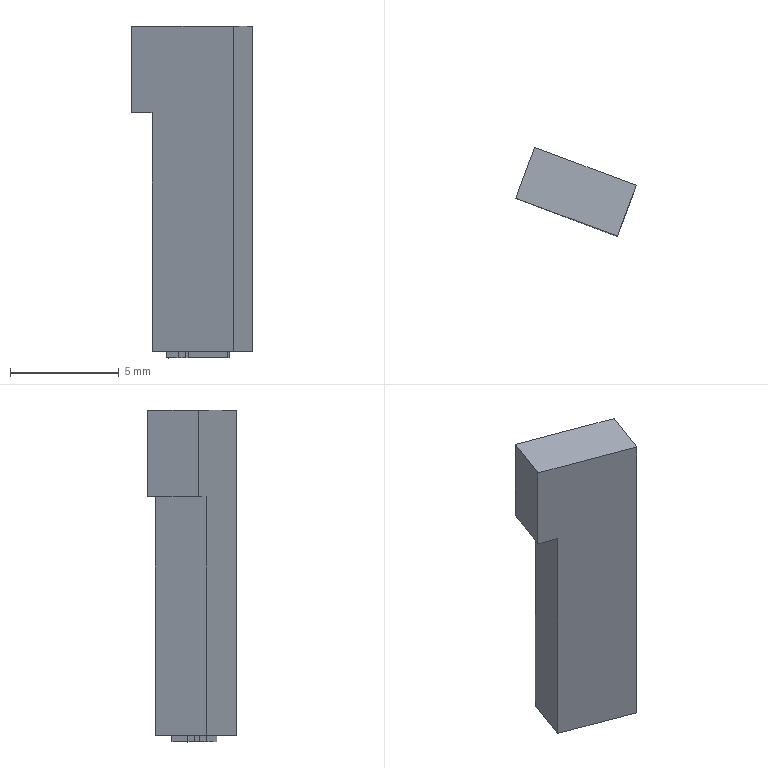Part | NX | features 13 2 | 1 solid | 24 faces | box 5.559 x 4.093 x 15.3 mm | volume 160.547 mm3 | plane 24
STEP:
#1=CARTESIAN_POINT('',(356.25,41.783,0.002111));
#2=VERTEX_POINT('',#1);
#3=CARTESIAN_POINT('',(355.374,39.441,0.002111));
#4=VERTEX_POINT('',#3);
#5=CARTESIAN_POINT('',(359.225,49.741,0.002111));
#6=DIRECTION('',(-0.3502,-0.9367,0.000000001));
#7=VECTOR('',#6,1000.);
#8=LINE('',#5,#7);
#9=EDGE_CURVE('',#2,#4,#8,.T.);
#10=ORIENTED_EDGE('',*,*,#9,.T.);
#11=CARTESIAN_POINT('',(351.627,40.842,0.002031));
#12=VERTEX_POINT('',#11);
#13=CARTESIAN_POINT('',(353.501,40.141,0.002071));
#14=DIRECTION('',(-0.9367,0.3502,-0.00001998));
#15=VECTOR('',#14,1000.);
#16=LINE('',#13,#15);
#17=EDGE_CURVE('',#4,#12,#16,.T.);
#18=ORIENTED_EDGE('',*,*,#17,.T.);
#19=CARTESIAN_POINT('',(352.503,43.183,0.002031));
#20=VERTEX_POINT('',#19);
#21=CARTESIAN_POINT('',(355.478,51.142,0.002031));
#22=DIRECTION('',(0.3502,0.9367,-0.000000001));
#23=VECTOR('',#22,1000.);
#24=LINE('',#21,#23);
#25=EDGE_CURVE('',#12,#20,#24,.T.);
#26=ORIENTED_EDGE('',*,*,#25,.T.);
#27=CARTESIAN_POINT('',(354.376,42.483,0.002071));
#28=DIRECTION('',(0.9367,-0.3502,0.00001998));
#29=VECTOR('',#28,1000.);
#30=LINE('',#27,#29);
#31=EDGE_CURVE('',#20,#2,#30,.T.);
#32=ORIENTED_EDGE('',*,*,#31,.T.);
#33=EDGE_LOOP('',(#10,#18,#26,#32));
#34=FACE_BOUND('',#33,.T.);
#35=CARTESIAN_POINT('',(352.297,41.392,0.00204));
#36=VERTEX_POINT('',#35);
#37=CARTESIAN_POINT('',(352.402,41.672,0.00204));
#38=VERTEX_POINT('',#37);
#39=CARTESIAN_POINT('',(355.885,50.989,0.00204));
#40=DIRECTION('',(0.3502,0.9367,-0.000000001));
#41=VECTOR('',#40,1000.);
#42=LINE('',#39,#41);
#43=EDGE_CURVE('',#36,#38,#42,.T.);
#44=ORIENTED_EDGE('',*,*,#43,.F.);
#45=CARTESIAN_POINT('',(352.97,41.141,0.002054));
#46=VERTEX_POINT('',#45);
#47=CARTESIAN_POINT('',(353.763,40.844,0.002071));
#48=DIRECTION('',(-0.9367,0.3502,-0.00001998));
#49=VECTOR('',#48,1000.);
#50=LINE('',#47,#49);
#51=EDGE_CURVE('',#46,#36,#50,.T.);
#52=ORIENTED_EDGE('',*,*,#51,.F.);
#53=CARTESIAN_POINT('',(352.855,40.833,0.002054));
#54=VERTEX_POINT('',#53);
#55=CARTESIAN_POINT('',(356.558,50.738,0.002054));
#56=DIRECTION('',(0.3502,0.9367,-0.000000001));
#57=VECTOR('',#56,1000.);
#58=LINE('',#55,#57);
#59=EDGE_CURVE('',#54,#46,#58,.T.);
#60=ORIENTED_EDGE('',*,*,#59,.F.);
#61=CARTESIAN_POINT('',(353.171,40.714,0.002061));
#62=VERTEX_POINT('',#61);
#63=CARTESIAN_POINT('',(353.648,40.536,0.002071));
#64=DIRECTION('',(-0.9367,0.3502,-0.00001998));
#65=VECTOR('',#64,1000.);
#66=LINE('',#63,#65);
#67=EDGE_CURVE('',#62,#54,#66,.T.);
#68=ORIENTED_EDGE('',*,*,#67,.F.);
#69=CARTESIAN_POINT('',(353.286,41.022,0.002061));
#70=VERTEX_POINT('',#69);
#71=CARTESIAN_POINT('',(356.874,50.62,0.002061));
#72=DIRECTION('',(-0.3502,-0.9367,0.000000001));
#73=VECTOR('',#72,1000.);
#74=LINE('',#71,#73);
#75=EDGE_CURVE('',#70,#62,#74,.T.);
#76=ORIENTED_EDGE('',*,*,#75,.F.);
#77=CARTESIAN_POINT('',(355.107,40.342,0.0021));
#78=VERTEX_POINT('',#77);
#79=CARTESIAN_POINT('',(353.763,40.844,0.002071));
#80=DIRECTION('',(-0.9367,0.3502,-0.00001998));
#81=VECTOR('',#80,1000.);
#82=LINE('',#79,#81);
#83=EDGE_CURVE('',#78,#70,#82,.T.);
#84=ORIENTED_EDGE('',*,*,#83,.F.);
#85=CARTESIAN_POINT('',(355.192,40.57,0.0021));
#86=VERTEX_POINT('',#85);
#87=CARTESIAN_POINT('',(358.695,49.939,0.0021));
#88=DIRECTION('',(-0.3502,-0.9367,0.000000001));
#89=VECTOR('',#88,1000.);
#90=LINE('',#87,#89);
#91=EDGE_CURVE('',#86,#78,#90,.T.);
#92=ORIENTED_EDGE('',*,*,#91,.F.);
#93=CARTESIAN_POINT('',(353.761,42.291,0.002061));
#94=VERTEX_POINT('',#93);
#95=CARTESIAN_POINT('',(351.223,45.342,0.001992));
#96=DIRECTION('',(0.6395,-0.7688,0.00001735));
#97=VECTOR('',#96,1000.);
#98=LINE('',#95,#97);
#99=EDGE_CURVE('',#94,#86,#98,.T.);
#100=ORIENTED_EDGE('',*,*,#99,.F.);
#101=CARTESIAN_POINT('',(353.444,42.41,0.002054));
#102=VERTEX_POINT('',#101);
#103=CARTESIAN_POINT('',(354.238,42.113,0.002071));
#104=DIRECTION('',(0.9367,-0.3502,0.00001998));
#105=VECTOR('',#104,1000.);
#106=LINE('',#103,#105);
#107=EDGE_CURVE('',#102,#94,#106,.T.);
#108=ORIENTED_EDGE('',*,*,#107,.F.);
#109=CARTESIAN_POINT('',(353.075,41.42,0.002054));
#110=VERTEX_POINT('',#109);
#111=CARTESIAN_POINT('',(356.558,50.738,0.002054));
#112=DIRECTION('',(0.3502,0.9367,-0.000000001));
#113=VECTOR('',#112,1000.);
#114=LINE('',#111,#113);
#115=EDGE_CURVE('',#110,#102,#114,.T.);
#116=ORIENTED_EDGE('',*,*,#115,.F.);
#117=CARTESIAN_POINT('',(353.868,41.124,0.002071));
#118=DIRECTION('',(0.9367,-0.3502,0.00001998));
#119=VECTOR('',#118,1000.);
#120=LINE('',#117,#119);
#121=EDGE_CURVE('',#38,#110,#120,.T.);
#122=ORIENTED_EDGE('',*,*,#121,.F.);
#123=EDGE_LOOP('',(#44,#52,#60,#68,#76,#84,#92,#100,#108,#116,#122));
#124=FACE_BOUND('',#123,.T.);
#125=CARTESIAN_POINT('',(357.352,50.441,0.002071));
#126=DIRECTION('',(-0.00001871,0.000006998,1.));
#127=DIRECTION('',(0.9172,-0.3985,0.00001995));
#128=AXIS2_PLACEMENT_3D('',#125,#126,#127);
#129=PLANE('',#128);
#130=ADVANCED_FACE('',(#34,#124),#129,.F.);
#131=CARTESIAN_POINT('',(351.627,40.842,11.002));
#132=VERTEX_POINT('',#131);
#133=CARTESIAN_POINT('',(352.503,43.184,11.002));
#134=VERTEX_POINT('',#133);
#135=CARTESIAN_POINT('',(352.503,43.184,11.002));
#136=DIRECTION('',(0.3502,0.9367,-0.000000001));
#137=VECTOR('',#136,1000.);
#138=LINE('',#135,#137);
#139=EDGE_CURVE('',#132,#134,#138,.T.);
#140=ORIENTED_EDGE('',*,*,#139,.F.);
#141=CARTESIAN_POINT('',(350.691,41.192,11.002));
#142=VERTEX_POINT('',#141);
#143=CARTESIAN_POINT('',(353.501,40.141,11.002));
#144=DIRECTION('',(-0.9367,0.3502,-0.00001998));
#145=VECTOR('',#144,1000.);
#146=LINE('',#143,#145);
#147=EDGE_CURVE('',#132,#142,#146,.T.);
#148=ORIENTED_EDGE('',*,*,#147,.T.);
#149=CARTESIAN_POINT('',(351.566,43.534,11.002));
#150=VERTEX_POINT('',#149);
#151=CARTESIAN_POINT('',(353.666,49.15,11.002));
#152=DIRECTION('',(-0.3502,-0.9367,0.000000001));
#153=VECTOR('',#152,1000.);
#154=LINE('',#151,#153);
#155=EDGE_CURVE('',#150,#142,#154,.T.);
#156=ORIENTED_EDGE('',*,*,#155,.F.);
#157=CARTESIAN_POINT('',(354.376,42.483,11.002));
#158=DIRECTION('',(-0.9367,0.3502,-0.00001998));
#159=VECTOR('',#158,1000.);
#160=LINE('',#157,#159);
#161=EDGE_CURVE('',#134,#150,#160,.T.);
#162=ORIENTED_EDGE('',*,*,#161,.F.);
#163=EDGE_LOOP('',(#140,#148,#156,#162));
#164=FACE_BOUND('',#163,.T.);
#165=CARTESIAN_POINT('',(356.476,48.1,11.002));
#166=DIRECTION('',(0.00001871,-0.000006998,-1.));
#167=DIRECTION('',(0.9367,-0.3502,0.00001998));
#168=AXIS2_PLACEMENT_3D('',#165,#166,#167);
#169=PLANE('',#168);
#170=ADVANCED_FACE('',(#164),#169,.T.);
#171=CARTESIAN_POINT('',(355.374,39.441,15.002));
#172=VERTEX_POINT('',#171);
#173=CARTESIAN_POINT('',(356.249,41.783,15.002));
#174=VERTEX_POINT('',#173);
#175=CARTESIAN_POINT('',(356.249,41.783,15.002));
#176=DIRECTION('',(0.3502,0.9367,-0.000000001));
#177=VECTOR('',#176,1000.);
#178=LINE('',#175,#177);
#179=EDGE_CURVE('',#172,#174,#178,.T.);
#180=ORIENTED_EDGE('',*,*,#179,.T.);
#181=CARTESIAN_POINT('',(351.566,43.534,15.002));
#182=VERTEX_POINT('',#181);
#183=CARTESIAN_POINT('',(354.376,42.483,15.002));
#184=DIRECTION('',(0.9367,-0.3502,0.00001998));
#185=VECTOR('',#184,1000.);
#186=LINE('',#183,#185);
#187=EDGE_CURVE('',#182,#174,#186,.T.);
#188=ORIENTED_EDGE('',*,*,#187,.F.);
#189=CARTESIAN_POINT('',(350.69,41.192,15.002));
#190=VERTEX_POINT('',#189);
#191=CARTESIAN_POINT('',(354.541,51.492,15.002));
#192=DIRECTION('',(-0.3502,-0.9367,0.000000001));
#193=VECTOR('',#192,1000.);
#194=LINE('',#191,#193);
#195=EDGE_CURVE('',#182,#190,#194,.T.);
#196=ORIENTED_EDGE('',*,*,#195,.T.);
#197=CARTESIAN_POINT('',(353.501,40.141,15.002));
#198=DIRECTION('',(-0.9367,0.3502,-0.00001998));
#199=VECTOR('',#198,1000.);
#200=LINE('',#197,#199);
#201=EDGE_CURVE('',#172,#190,#200,.T.);
#202=ORIENTED_EDGE('',*,*,#201,.F.);
#203=EDGE_LOOP('',(#180,#188,#196,#202));
#204=FACE_BOUND('',#203,.T.);
#205=CARTESIAN_POINT('',(357.351,50.441,15.002));
#206=DIRECTION('',(0.00001871,-0.000006998,-1.));
#207=DIRECTION('',(-0.9172,0.3985,-0.00001995));
#208=AXIS2_PLACEMENT_3D('',#205,#206,#207);
#209=PLANE('',#208);
#210=ADVANCED_FACE('',(#204),#209,.F.);
#211=CARTESIAN_POINT('',(355.374,39.441,-0.3542));
#212=DIRECTION('',(-0.00001871,0.000006998,1.));
#213=VECTOR('',#212,1000.);
#214=LINE('',#211,#213);
#215=EDGE_CURVE('',#4,#172,#214,.T.);
#216=ORIENTED_EDGE('',*,*,#215,.F.);
#217=ORIENTED_EDGE('',*,*,#9,.F.);
#218=CARTESIAN_POINT('',(356.25,41.783,-0.3522));
#219=DIRECTION('',(-0.00001871,0.000006998,1.));
#220=VECTOR('',#219,1000.);
#221=LINE('',#218,#220);
#222=EDGE_CURVE('',#2,#174,#221,.T.);
#223=ORIENTED_EDGE('',*,*,#222,.T.);
#224=ORIENTED_EDGE('',*,*,#179,.F.);
#225=EDGE_LOOP('',(#216,#217,#223,#224));
#226=FACE_BOUND('',#225,.T.);
#227=CARTESIAN_POINT('',(356.25,41.783,-0.3522));
#228=DIRECTION('',(-0.9367,0.3502,-0.00001998));
#229=DIRECTION('',(-0.3502,-0.9367,0.000000001));
#230=AXIS2_PLACEMENT_3D('',#227,#228,#229);
#231=PLANE('',#230);
#232=ADVANCED_FACE('',(#226),#231,.F.);
#233=ORIENTED_EDGE('',*,*,#222,.F.);
#234=ORIENTED_EDGE('',*,*,#31,.F.);
#235=CARTESIAN_POINT('',(352.503,43.183,-0.3524));
#236=DIRECTION('',(-0.00001871,0.000006998,1.));
#237=VECTOR('',#236,1000.);
#238=LINE('',#235,#237);
#239=EDGE_CURVE('',#20,#134,#238,.T.);
#240=ORIENTED_EDGE('',*,*,#239,.T.);
#241=ORIENTED_EDGE('',*,*,#161,.T.);
#242=CARTESIAN_POINT('',(351.566,43.534,-0.3524));
#243=DIRECTION('',(-0.00001871,0.000006998,1.));
#244=VECTOR('',#243,1000.);
#245=LINE('',#242,#244);
#246=EDGE_CURVE('',#150,#182,#245,.T.);
#247=ORIENTED_EDGE('',*,*,#246,.T.);
#248=ORIENTED_EDGE('',*,*,#187,.T.);
#249=EDGE_LOOP('',(#233,#234,#240,#241,#247,#248));
#250=FACE_BOUND('',#249,.T.);
#251=CARTESIAN_POINT('',(354.376,42.483,-0.3523));
#252=DIRECTION('',(-0.3502,-0.9367,0.000000001));
#253=DIRECTION('',(0.9367,-0.3502,0.00001998));
#254=AXIS2_PLACEMENT_3D('',#251,#252,#253);
#255=PLANE('',#254);
#256=ADVANCED_FACE('',(#250),#255,.F.);
#257=ORIENTED_EDGE('',*,*,#155,.T.);
#258=CARTESIAN_POINT('',(350.691,41.192,-0.3524));
#259=DIRECTION('',(-0.00001871,0.000006998,1.));
#260=VECTOR('',#259,1000.);
#261=LINE('',#258,#260);
#262=EDGE_CURVE('',#142,#190,#261,.T.);
#263=ORIENTED_EDGE('',*,*,#262,.T.);
#264=ORIENTED_EDGE('',*,*,#195,.F.);
#265=ORIENTED_EDGE('',*,*,#246,.F.);
#266=EDGE_LOOP('',(#257,#263,#264,#265));
#267=FACE_BOUND('',#266,.T.);
#268=CARTESIAN_POINT('',(351.566,43.534,-0.3524));
#269=DIRECTION('',(0.9367,-0.3502,0.00001998));
#270=DIRECTION('',(0.3502,0.9367,-0.000000001));
#271=AXIS2_PLACEMENT_3D('',#268,#269,#270);
#272=PLANE('',#271);
#273=ADVANCED_FACE('',(#267),#272,.F.);
#274=ORIENTED_EDGE('',*,*,#147,.F.);
#275=CARTESIAN_POINT('',(351.627,40.842,-0.3543));
#276=DIRECTION('',(-0.00001871,0.000006998,1.));
#277=VECTOR('',#276,1000.);
#278=LINE('',#275,#277);
#279=EDGE_CURVE('',#12,#132,#278,.T.);
#280=ORIENTED_EDGE('',*,*,#279,.F.);
#281=ORIENTED_EDGE('',*,*,#17,.F.);
#282=ORIENTED_EDGE('',*,*,#215,.T.);
#283=ORIENTED_EDGE('',*,*,#201,.T.);
#284=ORIENTED_EDGE('',*,*,#262,.F.);
#285=EDGE_LOOP('',(#274,#280,#281,#282,#283,#284));
#286=FACE_BOUND('',#285,.T.);
#287=CARTESIAN_POINT('',(353.501,40.141,-0.3543));
#288=DIRECTION('',(0.3502,0.9367,-0.000000001));
#289=DIRECTION('',(-0.9367,0.3502,-0.00001998));
#290=AXIS2_PLACEMENT_3D('',#287,#288,#289);
#291=PLANE('',#290);
#292=ADVANCED_FACE('',(#286),#291,.F.);
#293=ORIENTED_EDGE('',*,*,#279,.T.);
#294=ORIENTED_EDGE('',*,*,#139,.T.);
#295=ORIENTED_EDGE('',*,*,#239,.F.);
#296=ORIENTED_EDGE('',*,*,#25,.F.);
#297=EDGE_LOOP('',(#293,#294,#295,#296));
#298=FACE_BOUND('',#297,.T.);
#299=CARTESIAN_POINT('',(352.503,43.183,-0.3524));
#300=DIRECTION('',(0.9367,-0.3502,0.00001998));
#301=DIRECTION('',(0.3502,0.9367,-0.000000001));
#302=AXIS2_PLACEMENT_3D('',#299,#300,#301);
#303=PLANE('',#302);
#304=ADVANCED_FACE('',(#298),#303,.F.);
#305=CARTESIAN_POINT('',(353.658,42.016,-0.298));
#306=VERTEX_POINT('',#305);
#307=CARTESIAN_POINT('',(353.658,42.016,0.002061));
#308=VERTEX_POINT('',#307);
#309=CARTESIAN_POINT('',(353.658,42.016,-14.998));
#310=DIRECTION('',(-0.00001871,0.000006998,1.));
#311=VECTOR('',#310,1000.);
#312=LINE('',#309,#311);
#313=EDGE_CURVE('',#306,#308,#312,.T.);
#314=ORIENTED_EDGE('',*,*,#313,.T.);
#315=CARTESIAN_POINT('',(353.391,41.302,0.002061));
#316=VERTEX_POINT('',#315);
#317=CARTESIAN_POINT('',(356.874,50.62,0.002061));
#318=DIRECTION('',(-0.3502,-0.9367,0.000000001));
#319=VECTOR('',#318,1000.);
#320=LINE('',#317,#319);
#321=EDGE_CURVE('',#308,#316,#320,.T.);
#322=ORIENTED_EDGE('',*,*,#321,.T.);
#323=CARTESIAN_POINT('',(353.391,41.302,-0.298));
#324=VERTEX_POINT('',#323);
#325=CARTESIAN_POINT('',(353.391,41.302,-14.998));
#326=DIRECTION('',(-0.00001871,0.000006998,1.));
#327=VECTOR('',#326,1000.);
#328=LINE('',#325,#327);
#329=EDGE_CURVE('',#324,#316,#328,.T.);
#330=ORIENTED_EDGE('',*,*,#329,.F.);
#331=CARTESIAN_POINT('',(357.615,52.599,-0.298));
#332=DIRECTION('',(-0.3502,-0.9367,0.000000001));
#333=VECTOR('',#332,1000.);
#334=LINE('',#331,#333);
#335=EDGE_CURVE('',#306,#324,#334,.T.);
#336=ORIENTED_EDGE('',*,*,#335,.F.);
#337=EDGE_LOOP('',(#314,#322,#330,#336));
#338=FACE_BOUND('',#337,.T.);
#339=CARTESIAN_POINT('',(353.658,42.016,-14.998));
#340=DIRECTION('',(-0.9367,0.3502,-0.00001998));
#341=DIRECTION('',(-0.3502,-0.9367,0.000000001));
#342=AXIS2_PLACEMENT_3D('',#339,#340,#341);
#343=PLANE('',#342);
#344=ADVANCED_FACE('',(#338),#343,.F.);
#345=ORIENTED_EDGE('',*,*,#329,.T.);
#346=CARTESIAN_POINT('',(354.657,40.829,0.002088));
#347=VERTEX_POINT('',#346);
#348=CARTESIAN_POINT('',(353.868,41.124,0.002071));
#349=DIRECTION('',(0.9367,-0.3502,0.00001998));
#350=VECTOR('',#349,1000.);
#351=LINE('',#348,#350);
#352=EDGE_CURVE('',#316,#347,#351,.T.);
#353=ORIENTED_EDGE('',*,*,#352,.T.);
#354=CARTESIAN_POINT('',(354.657,40.829,-0.2979));
#355=VERTEX_POINT('',#354);
#356=CARTESIAN_POINT('',(354.658,40.829,-14.998));
#357=DIRECTION('',(-0.00001871,0.000006998,1.));
#358=VECTOR('',#357,1000.);
#359=LINE('',#356,#358);
#360=EDGE_CURVE('',#355,#347,#359,.T.);
#361=ORIENTED_EDGE('',*,*,#360,.F.);
#362=CARTESIAN_POINT('',(357.036,39.939,-0.2979));
#363=DIRECTION('',(0.9367,-0.3502,0.00001998));
#364=VECTOR('',#363,1000.);
#365=LINE('',#362,#364);
#366=EDGE_CURVE('',#324,#355,#365,.T.);
#367=ORIENTED_EDGE('',*,*,#366,.F.);
#368=EDGE_LOOP('',(#345,#353,#361,#367));
#369=FACE_BOUND('',#368,.T.);
#370=CARTESIAN_POINT('',(353.391,41.302,-14.998));
#371=DIRECTION('',(-0.3502,-0.9367,0.000000001));
#372=DIRECTION('',(0.9367,-0.3502,0.00001998));
#373=AXIS2_PLACEMENT_3D('',#370,#371,#372);
#374=PLANE('',#373);
#375=ADVANCED_FACE('',(#369),#374,.F.);
#376=CARTESIAN_POINT('',(352.297,41.392,-0.298));
#377=VERTEX_POINT('',#376);
#378=CARTESIAN_POINT('',(352.297,41.392,-14.998));
#379=DIRECTION('',(-0.00001871,0.000006998,1.));
#380=VECTOR('',#379,1000.);
#381=LINE('',#378,#380);
#382=EDGE_CURVE('',#377,#36,#381,.T.);
#383=ORIENTED_EDGE('',*,*,#382,.T.);
#384=ORIENTED_EDGE('',*,*,#43,.T.);
#385=CARTESIAN_POINT('',(352.402,41.672,-0.298));
#386=VERTEX_POINT('',#385);
#387=CARTESIAN_POINT('',(352.402,41.672,-14.998));
#388=DIRECTION('',(-0.00001871,0.000006998,1.));
#389=VECTOR('',#388,1000.);
#390=LINE('',#387,#389);
#391=EDGE_CURVE('',#386,#38,#390,.T.);
#392=ORIENTED_EDGE('',*,*,#391,.F.);
#393=CARTESIAN_POINT('',(356.625,52.969,-0.298));
#394=DIRECTION('',(0.3502,0.9367,-0.000000001));
#395=VECTOR('',#394,1000.);
#396=LINE('',#393,#395);
#397=EDGE_CURVE('',#377,#386,#396,.T.);
#398=ORIENTED_EDGE('',*,*,#397,.F.);
#399=EDGE_LOOP('',(#383,#384,#392,#398));
#400=FACE_BOUND('',#399,.T.);
#401=CARTESIAN_POINT('',(352.297,41.392,-14.998));
#402=DIRECTION('',(0.9367,-0.3502,0.00001998));
#403=DIRECTION('',(0.3502,0.9367,-0.000000001));
#404=AXIS2_PLACEMENT_3D('',#401,#402,#403);
#405=PLANE('',#404);
#406=ADVANCED_FACE('',(#400),#405,.F.);
#407=ORIENTED_EDGE('',*,*,#391,.T.);
#408=ORIENTED_EDGE('',*,*,#121,.T.);
#409=CARTESIAN_POINT('',(353.075,41.42,-0.298));
#410=VERTEX_POINT('',#409);
#411=CARTESIAN_POINT('',(353.075,41.42,-14.998));
#412=DIRECTION('',(-0.00001871,0.000006998,1.));
#413=VECTOR('',#412,1000.);
#414=LINE('',#411,#413);
#415=EDGE_CURVE('',#410,#110,#414,.T.);
#416=ORIENTED_EDGE('',*,*,#415,.F.);
#417=CARTESIAN_POINT('',(357.036,39.939,-0.2979));
#418=DIRECTION('',(0.9367,-0.3502,0.00001998));
#419=VECTOR('',#418,1000.);
#420=LINE('',#417,#419);
#421=EDGE_CURVE('',#386,#410,#420,.T.);
#422=ORIENTED_EDGE('',*,*,#421,.F.);
#423=EDGE_LOOP('',(#407,#408,#416,#422));
#424=FACE_BOUND('',#423,.T.);
#425=CARTESIAN_POINT('',(352.402,41.672,-14.998));
#426=DIRECTION('',(-0.3502,-0.9367,0.000000001));
#427=DIRECTION('',(0.9367,-0.3502,0.00001998));
#428=AXIS2_PLACEMENT_3D('',#425,#426,#427);
#429=PLANE('',#428);
#430=ADVANCED_FACE('',(#424),#429,.F.);
#431=ORIENTED_EDGE('',*,*,#415,.T.);
#432=ORIENTED_EDGE('',*,*,#115,.T.);
#433=CARTESIAN_POINT('',(353.444,42.41,-0.298));
#434=VERTEX_POINT('',#433);
#435=CARTESIAN_POINT('',(353.445,42.409,-14.998));
#436=DIRECTION('',(-0.00001871,0.000006998,1.));
#437=VECTOR('',#436,1000.);
#438=LINE('',#435,#437);
#439=EDGE_CURVE('',#434,#102,#438,.T.);
#440=ORIENTED_EDGE('',*,*,#439,.F.);
#441=CARTESIAN_POINT('',(357.298,52.718,-0.298));
#442=DIRECTION('',(0.3502,0.9367,-0.000000001));
#443=VECTOR('',#442,1000.);
#444=LINE('',#441,#443);
#445=EDGE_CURVE('',#410,#434,#444,.T.);
#446=ORIENTED_EDGE('',*,*,#445,.F.);
#447=EDGE_LOOP('',(#431,#432,#440,#446));
#448=FACE_BOUND('',#447,.T.);
#449=CARTESIAN_POINT('',(353.075,41.42,-14.998));
#450=DIRECTION('',(0.9367,-0.3502,0.00001998));
#451=DIRECTION('',(0.3502,0.9367,-0.000000001));
#452=AXIS2_PLACEMENT_3D('',#449,#450,#451);
#453=PLANE('',#452);
#454=ADVANCED_FACE('',(#448),#453,.F.);
#455=ORIENTED_EDGE('',*,*,#439,.T.);
#456=ORIENTED_EDGE('',*,*,#107,.T.);
#457=CARTESIAN_POINT('',(353.761,42.291,-0.298));
#458=VERTEX_POINT('',#457);
#459=CARTESIAN_POINT('',(353.761,42.291,-14.998));
#460=DIRECTION('',(-0.00001871,0.000006998,1.));
#461=VECTOR('',#460,1000.);
#462=LINE('',#459,#461);
#463=EDGE_CURVE('',#458,#94,#462,.T.);
#464=ORIENTED_EDGE('',*,*,#463,.F.);
#465=CARTESIAN_POINT('',(357.406,40.929,-0.2979));
#466=DIRECTION('',(0.9367,-0.3502,0.00001998));
#467=VECTOR('',#466,1000.);
#468=LINE('',#465,#467);
#469=EDGE_CURVE('',#434,#458,#468,.T.);
#470=ORIENTED_EDGE('',*,*,#469,.F.);
#471=EDGE_LOOP('',(#455,#456,#464,#470));
#472=FACE_BOUND('',#471,.T.);
#473=CARTESIAN_POINT('',(353.445,42.409,-14.998));
#474=DIRECTION('',(-0.3502,-0.9367,0.000000001));
#475=DIRECTION('',(0.9367,-0.3502,0.00001998));
#476=AXIS2_PLACEMENT_3D('',#473,#474,#475);
#477=PLANE('',#476);
#478=ADVANCED_FACE('',(#472),#477,.F.);
#479=ORIENTED_EDGE('',*,*,#463,.T.);
#480=ORIENTED_EDGE('',*,*,#99,.T.);
#481=CARTESIAN_POINT('',(355.192,40.57,-0.2979));
#482=VERTEX_POINT('',#481);
#483=CARTESIAN_POINT('',(355.193,40.57,-14.998));
#484=DIRECTION('',(-0.00001871,0.000006998,1.));
#485=VECTOR('',#484,1000.);
#486=LINE('',#483,#485);
#487=EDGE_CURVE('',#482,#86,#486,.T.);
#488=ORIENTED_EDGE('',*,*,#487,.F.);
#489=CARTESIAN_POINT('',(352.43,43.891,-0.298));
#490=DIRECTION('',(0.6395,-0.7688,0.00001735));
#491=VECTOR('',#490,1000.);
#492=LINE('',#489,#491);
#493=EDGE_CURVE('',#458,#482,#492,.T.);
#494=ORIENTED_EDGE('',*,*,#493,.F.);
#495=EDGE_LOOP('',(#479,#480,#488,#494));
#496=FACE_BOUND('',#495,.T.);
#497=CARTESIAN_POINT('',(353.761,42.291,-14.998));
#498=DIRECTION('',(-0.7688,-0.6395,-0.000009911));
#499=DIRECTION('',(0.6395,-0.7688,0.00001735));
#500=AXIS2_PLACEMENT_3D('',#497,#498,#499);
#501=PLANE('',#500);
#502=ADVANCED_FACE('',(#496),#501,.F.);
#503=ORIENTED_EDGE('',*,*,#487,.T.);
#504=ORIENTED_EDGE('',*,*,#91,.T.);
#505=CARTESIAN_POINT('',(355.107,40.342,-0.2979));
#506=VERTEX_POINT('',#505);
#507=CARTESIAN_POINT('',(355.107,40.341,-14.998));
#508=DIRECTION('',(-0.00001871,0.000006998,1.));
#509=VECTOR('',#508,1000.);
#510=LINE('',#507,#509);
#511=EDGE_CURVE('',#506,#78,#510,.T.);
#512=ORIENTED_EDGE('',*,*,#511,.F.);
#513=CARTESIAN_POINT('',(359.435,51.919,-0.2979));
#514=DIRECTION('',(-0.3502,-0.9367,0.000000001));
#515=VECTOR('',#514,1000.);
#516=LINE('',#513,#515);
#517=EDGE_CURVE('',#482,#506,#516,.T.);
#518=ORIENTED_EDGE('',*,*,#517,.F.);
#519=EDGE_LOOP('',(#503,#504,#512,#518));
#520=FACE_BOUND('',#519,.T.);
#521=CARTESIAN_POINT('',(355.193,40.57,-14.998));
#522=DIRECTION('',(-0.9367,0.3502,-0.00001998));
#523=DIRECTION('',(-0.3502,-0.9367,0.000000001));
#524=AXIS2_PLACEMENT_3D('',#521,#522,#523);
#525=PLANE('',#524);
#526=ADVANCED_FACE('',(#520),#525,.F.);
#527=ORIENTED_EDGE('',*,*,#511,.T.);
#528=ORIENTED_EDGE('',*,*,#83,.T.);
#529=CARTESIAN_POINT('',(353.286,41.022,-0.298));
#530=VERTEX_POINT('',#529);
#531=CARTESIAN_POINT('',(353.286,41.022,-14.998));
#532=DIRECTION('',(-0.00001871,0.000006998,1.));
#533=VECTOR('',#532,1000.);
#534=LINE('',#531,#533);
#535=EDGE_CURVE('',#530,#70,#534,.T.);
#536=ORIENTED_EDGE('',*,*,#535,.F.);
#537=CARTESIAN_POINT('',(356.931,39.659,-0.2979));
#538=DIRECTION('',(-0.9367,0.3502,-0.00001998));
#539=VECTOR('',#538,1000.);
#540=LINE('',#537,#539);
#541=EDGE_CURVE('',#506,#530,#540,.T.);
#542=ORIENTED_EDGE('',*,*,#541,.F.);
#543=EDGE_LOOP('',(#527,#528,#536,#542));
#544=FACE_BOUND('',#543,.T.);
#545=CARTESIAN_POINT('',(355.107,40.341,-14.998));
#546=DIRECTION('',(0.3502,0.9367,-0.000000001));
#547=DIRECTION('',(-0.9367,0.3502,-0.00001998));
#548=AXIS2_PLACEMENT_3D('',#545,#546,#547);
#549=PLANE('',#548);
#550=ADVANCED_FACE('',(#544),#549,.F.);
#551=ORIENTED_EDGE('',*,*,#535,.T.);
#552=ORIENTED_EDGE('',*,*,#75,.T.);
#553=CARTESIAN_POINT('',(353.171,40.714,-0.298));
#554=VERTEX_POINT('',#553);
#555=CARTESIAN_POINT('',(353.171,40.714,-14.998));
#556=DIRECTION('',(-0.00001871,0.000006998,1.));
#557=VECTOR('',#556,1000.);
#558=LINE('',#555,#557);
#559=EDGE_CURVE('',#554,#62,#558,.T.);
#560=ORIENTED_EDGE('',*,*,#559,.F.);
#561=CARTESIAN_POINT('',(357.615,52.599,-0.298));
#562=DIRECTION('',(-0.3502,-0.9367,0.000000001));
#563=VECTOR('',#562,1000.);
#564=LINE('',#561,#563);
#565=EDGE_CURVE('',#530,#554,#564,.T.);
#566=ORIENTED_EDGE('',*,*,#565,.F.);
#567=EDGE_LOOP('',(#551,#552,#560,#566));
#568=FACE_BOUND('',#567,.T.);
#569=CARTESIAN_POINT('',(353.286,41.022,-14.998));
#570=DIRECTION('',(-0.9367,0.3502,-0.00001998));
#571=DIRECTION('',(-0.3502,-0.9367,0.000000001));
#572=AXIS2_PLACEMENT_3D('',#569,#570,#571);
#573=PLANE('',#572);
#574=ADVANCED_FACE('',(#568),#573,.F.);
#575=ORIENTED_EDGE('',*,*,#559,.T.);
#576=ORIENTED_EDGE('',*,*,#67,.T.);
#577=CARTESIAN_POINT('',(352.855,40.833,-0.298));
#578=VERTEX_POINT('',#577);
#579=CARTESIAN_POINT('',(352.855,40.833,-14.998));
#580=DIRECTION('',(-0.00001871,0.000006998,1.));
#581=VECTOR('',#580,1000.);
#582=LINE('',#579,#581);
#583=EDGE_CURVE('',#578,#54,#582,.T.);
#584=ORIENTED_EDGE('',*,*,#583,.F.);
#585=CARTESIAN_POINT('',(356.816,39.352,-0.2979));
#586=DIRECTION('',(-0.9367,0.3502,-0.00001998));
#587=VECTOR('',#586,1000.);
#588=LINE('',#585,#587);
#589=EDGE_CURVE('',#554,#578,#588,.T.);
#590=ORIENTED_EDGE('',*,*,#589,.F.);
#591=EDGE_LOOP('',(#575,#576,#584,#590));
#592=FACE_BOUND('',#591,.T.);
#593=CARTESIAN_POINT('',(353.171,40.714,-14.998));
#594=DIRECTION('',(0.3502,0.9367,-0.000000001));
#595=DIRECTION('',(-0.9367,0.3502,-0.00001998));
#596=AXIS2_PLACEMENT_3D('',#593,#594,#595);
#597=PLANE('',#596);
#598=ADVANCED_FACE('',(#592),#597,.F.);
#599=ORIENTED_EDGE('',*,*,#583,.T.);
#600=ORIENTED_EDGE('',*,*,#59,.T.);
#601=CARTESIAN_POINT('',(352.97,41.141,-0.298));
#602=VERTEX_POINT('',#601);
#603=CARTESIAN_POINT('',(352.97,41.14,-14.998));
#604=DIRECTION('',(-0.00001871,0.000006998,1.));
#605=VECTOR('',#604,1000.);
#606=LINE('',#603,#605);
#607=EDGE_CURVE('',#602,#46,#606,.T.);
#608=ORIENTED_EDGE('',*,*,#607,.F.);
#609=CARTESIAN_POINT('',(357.298,52.718,-0.298));
#610=DIRECTION('',(0.3502,0.9367,-0.000000001));
#611=VECTOR('',#610,1000.);
#612=LINE('',#609,#611);
#613=EDGE_CURVE('',#578,#602,#612,.T.);
#614=ORIENTED_EDGE('',*,*,#613,.F.);
#615=EDGE_LOOP('',(#599,#600,#608,#614));
#616=FACE_BOUND('',#615,.T.);
#617=CARTESIAN_POINT('',(352.855,40.833,-14.998));
#618=DIRECTION('',(0.9367,-0.3502,0.00001998));
#619=DIRECTION('',(0.3502,0.9367,-0.000000001));
#620=AXIS2_PLACEMENT_3D('',#617,#618,#619);
#621=PLANE('',#620);
#622=ADVANCED_FACE('',(#616),#621,.F.);
#623=ORIENTED_EDGE('',*,*,#607,.T.);
#624=ORIENTED_EDGE('',*,*,#51,.T.);
#625=ORIENTED_EDGE('',*,*,#382,.F.);
#626=CARTESIAN_POINT('',(356.931,39.659,-0.2979));
#627=DIRECTION('',(-0.9367,0.3502,-0.00001998));
#628=VECTOR('',#627,1000.);
#629=LINE('',#626,#628);
#630=EDGE_CURVE('',#602,#377,#629,.T.);
#631=ORIENTED_EDGE('',*,*,#630,.F.);
#632=EDGE_LOOP('',(#623,#624,#625,#631));
#633=FACE_BOUND('',#632,.T.);
#634=CARTESIAN_POINT('',(352.97,41.14,-14.998));
#635=DIRECTION('',(0.3502,0.9367,-0.000000001));
#636=DIRECTION('',(-0.9367,0.3502,-0.00001998));
#637=AXIS2_PLACEMENT_3D('',#634,#635,#636);
#638=PLANE('',#637);
#639=ADVANCED_FACE('',(#633),#638,.F.);
#640=ORIENTED_EDGE('',*,*,#360,.T.);
#641=CARTESIAN_POINT('',(351.039,45.126,0.00199));
#642=DIRECTION('',(-0.6441,0.765,-0.00001741));
#643=VECTOR('',#642,1000.);
#644=LINE('',#641,#643);
#645=EDGE_CURVE('',#347,#308,#644,.T.);
#646=ORIENTED_EDGE('',*,*,#645,.T.);
#647=ORIENTED_EDGE('',*,*,#313,.F.);
#648=CARTESIAN_POINT('',(352.268,43.666,-0.298));
#649=DIRECTION('',(-0.6441,0.765,-0.00001741));
#650=VECTOR('',#649,1000.);
#651=LINE('',#648,#650);
#652=EDGE_CURVE('',#355,#306,#651,.T.);
#653=ORIENTED_EDGE('',*,*,#652,.F.);
#654=EDGE_LOOP('',(#640,#646,#647,#653));
#655=FACE_BOUND('',#654,.T.);
#656=CARTESIAN_POINT('',(354.658,40.829,-14.998));
#657=DIRECTION('',(0.765,0.6441,0.000009809));
#658=DIRECTION('',(-0.6441,0.765,-0.00001741));
#659=AXIS2_PLACEMENT_3D('',#656,#657,#658);
#660=PLANE('',#659);
#661=ADVANCED_FACE('',(#655),#660,.F.);
#662=ORIENTED_EDGE('',*,*,#397,.T.);
#663=ORIENTED_EDGE('',*,*,#421,.T.);
#664=ORIENTED_EDGE('',*,*,#445,.T.);
#665=ORIENTED_EDGE('',*,*,#469,.T.);
#666=ORIENTED_EDGE('',*,*,#493,.T.);
#667=ORIENTED_EDGE('',*,*,#517,.T.);
#668=ORIENTED_EDGE('',*,*,#541,.T.);
#669=ORIENTED_EDGE('',*,*,#565,.T.);
#670=ORIENTED_EDGE('',*,*,#589,.T.);
#671=ORIENTED_EDGE('',*,*,#613,.T.);
#672=ORIENTED_EDGE('',*,*,#630,.T.);
#673=EDGE_LOOP('',(#662,#663,#664,#665,#666,#667,#668,#669,#670,#671,#672));
#674=FACE_BOUND('',#673,.T.);
#675=ORIENTED_EDGE('',*,*,#335,.T.);
#676=ORIENTED_EDGE('',*,*,#366,.T.);
#677=ORIENTED_EDGE('',*,*,#652,.T.);
#678=EDGE_LOOP('',(#675,#676,#677));
#679=FACE_BOUND('',#678,.T.);
#680=CARTESIAN_POINT('',(361.26,51.237,-0.2979));
#681=DIRECTION('',(-0.00001871,0.000006998,1.));
#682=DIRECTION('',(0.9367,-0.3502,0.00001998));
#683=AXIS2_PLACEMENT_3D('',#680,#681,#682);
#684=PLANE('',#683);
#685=ADVANCED_FACE('',(#674,#679),#684,.F.);
#686=ORIENTED_EDGE('',*,*,#321,.F.);
#687=ORIENTED_EDGE('',*,*,#645,.F.);
#688=ORIENTED_EDGE('',*,*,#352,.F.);
#689=EDGE_LOOP('',(#686,#687,#688));
#690=FACE_BOUND('',#689,.T.);
#691=CARTESIAN_POINT('',(357.352,50.441,0.002071));
#692=DIRECTION('',(-0.00001871,0.000006998,1.));
#693=DIRECTION('',(0.9172,-0.3985,0.00001995));
#694=AXIS2_PLACEMENT_3D('',#691,#692,#693);
#695=PLANE('',#694);
#696=ADVANCED_FACE('',(#690),#695,.F.);
#697=CLOSED_SHELL('',(#130,#170,#210,#232,#256,#273,#292,#304,#344,#375,#406,#430,#454,#478,#502,#526,#550,#574,#598,#622,#639,#661,#685,#696));
#698=MANIFOLD_SOLID_BREP('',#697);
#699=(LENGTH_UNIT()NAMED_UNIT(*)SI_UNIT(.MILLI.,.METRE.));
#700=UNCERTAINTY_MEASURE_WITH_UNIT(LENGTH_MEASURE(0.00001),#699,'','');
#701=(NAMED_UNIT(*)PLANE_ANGLE_UNIT()SI_UNIT($,.RADIAN.));
#702=(NAMED_UNIT(*)SI_UNIT($,.STERADIAN.)SOLID_ANGLE_UNIT());
#703=(GEOMETRIC_REPRESENTATION_CONTEXT(3)GLOBAL_UNCERTAINTY_ASSIGNED_CONTEXT((#700))GLOBAL_UNIT_ASSIGNED_CONTEXT((#699,#701,#702))REPRESENTATION_CONTEXT('',''));
#704=ADVANCED_BREP_SHAPE_REPRESENTATION('',(#698),#703);